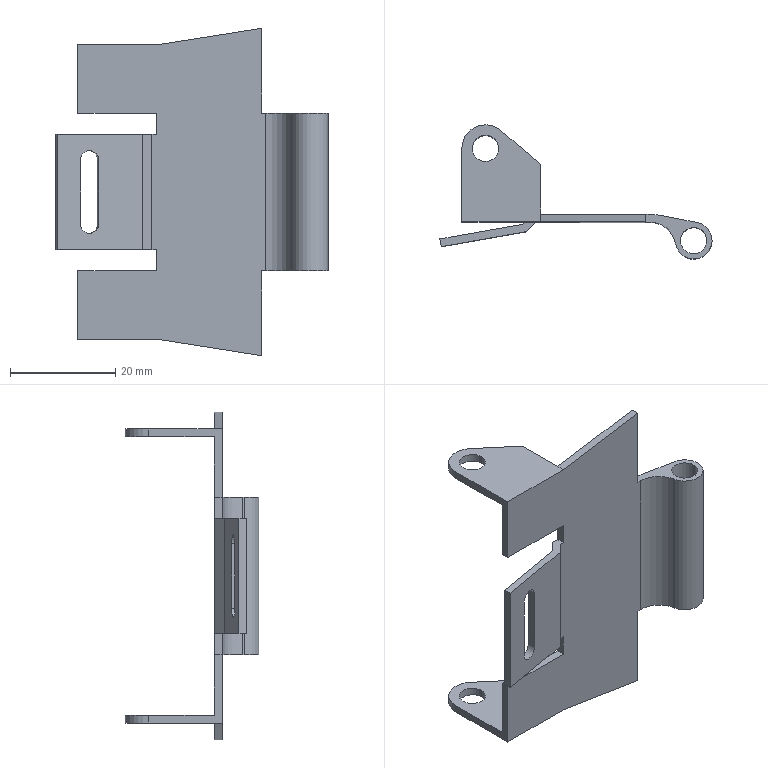Part | SolidWorks | features BaseBody 1 | 1 solid | 46 faces | box 51.82 x 25.52 x 62.335 mm | volume 4576 mm3 | plane 33 | cylinder 13 | commonest cylinder face diameters 5 x6 3.5 x2 9 x2 7 x1 10 x1 20 x1
STEP:
#1=CARTESIAN_POINT('',(2.5,0.,-1.5));
#2=VERTEX_POINT('',#1);
#3=CARTESIAN_POINT('',(-2.5,0.,-1.5));
#4=VERTEX_POINT('',#3);
#5=CARTESIAN_POINT('',(0.,0.,-1.5));
#6=DIRECTION('',(0.,0.,-1.));
#7=DIRECTION('',(1.,0.,0.));
#8=AXIS2_PLACEMENT_3D('',#5,#6,#7);
#9=CIRCLE('',#8,2.5);
#10=EDGE_CURVE('',#2,#4,#9,.T.);
#11=ORIENTED_EDGE('',*,*,#10,.T.);
#12=CARTESIAN_POINT('',(-2.5,0.,0.));
#13=VERTEX_POINT('',#12);
#14=CARTESIAN_POINT('',(-2.5,0.,-1.5));
#15=DIRECTION('',(0.,0.,1.));
#16=VECTOR('',#15,1000.);
#17=LINE('',#14,#16);
#18=EDGE_CURVE('',#4,#13,#17,.T.);
#19=ORIENTED_EDGE('',*,*,#18,.T.);
#20=CARTESIAN_POINT('',(2.5,0.,0.));
#21=VERTEX_POINT('',#20);
#22=CARTESIAN_POINT('',(0.,0.,0.));
#23=DIRECTION('',(0.,0.,-1.));
#24=DIRECTION('',(1.,0.,0.));
#25=AXIS2_PLACEMENT_3D('',#22,#23,#24);
#26=CIRCLE('',#25,2.5);
#27=EDGE_CURVE('',#21,#13,#26,.T.);
#28=ORIENTED_EDGE('',*,*,#27,.F.);
#29=CARTESIAN_POINT('',(2.5,0.,-1.5));
#30=DIRECTION('',(0.,0.,1.));
#31=VECTOR('',#30,1000.);
#32=LINE('',#29,#31);
#33=EDGE_CURVE('',#2,#21,#32,.T.);
#34=ORIENTED_EDGE('',*,*,#33,.F.);
#35=EDGE_LOOP('',(#11,#19,#28,#34));
#36=FACE_OUTER_BOUND('',#35,.T.);
#37=CARTESIAN_POINT('',(0.,0.,-1.5));
#38=DIRECTION('',(0.,0.,1.));
#39=DIRECTION('',(1.,0.,0.));
#40=AXIS2_PLACEMENT_3D('',#37,#38,#39);
#41=CYLINDRICAL_SURFACE('',#40,2.5);
#42=ADVANCED_FACE('',(#36),#41,.F.);
#43=CARTESIAN_POINT('',(2.5,0.,-54.5));
#44=VERTEX_POINT('',#43);
#45=CARTESIAN_POINT('',(-2.5,0.,-54.5));
#46=VERTEX_POINT('',#45);
#47=CARTESIAN_POINT('',(0.,0.,-54.5));
#48=DIRECTION('',(0.,0.,-1.));
#49=DIRECTION('',(-1.,0.,0.));
#50=AXIS2_PLACEMENT_3D('',#47,#48,#49);
#51=CIRCLE('',#50,2.5);
#52=EDGE_CURVE('',#44,#46,#51,.T.);
#53=ORIENTED_EDGE('',*,*,#52,.F.);
#54=CARTESIAN_POINT('',(2.5,0.,-56.));
#55=VERTEX_POINT('',#54);
#56=CARTESIAN_POINT('',(2.5,0.,-54.5));
#57=DIRECTION('',(0.,0.,-1.));
#58=VECTOR('',#57,1000.);
#59=LINE('',#56,#58);
#60=EDGE_CURVE('',#44,#55,#59,.T.);
#61=ORIENTED_EDGE('',*,*,#60,.T.);
#62=CARTESIAN_POINT('',(-2.5,0.,-56.));
#63=VERTEX_POINT('',#62);
#64=CARTESIAN_POINT('',(0.,0.,-56.));
#65=DIRECTION('',(0.,0.,1.));
#66=DIRECTION('',(-1.,0.,0.));
#67=AXIS2_PLACEMENT_3D('',#64,#65,#66);
#68=CIRCLE('',#67,2.5);
#69=EDGE_CURVE('',#63,#55,#68,.T.);
#70=ORIENTED_EDGE('',*,*,#69,.F.);
#71=CARTESIAN_POINT('',(-2.5,0.,-54.5));
#72=DIRECTION('',(0.,0.,-1.));
#73=VECTOR('',#72,1000.);
#74=LINE('',#71,#73);
#75=EDGE_CURVE('',#46,#63,#74,.T.);
#76=ORIENTED_EDGE('',*,*,#75,.F.);
#77=EDGE_LOOP('',(#53,#61,#70,#76));
#78=FACE_OUTER_BOUND('',#77,.T.);
#79=CARTESIAN_POINT('',(0.,0.,-54.5));
#80=DIRECTION('',(0.,0.,-1.));
#81=DIRECTION('',(-1.,0.,0.));
#82=AXIS2_PLACEMENT_3D('',#79,#80,#81);
#83=CYLINDRICAL_SURFACE('',#82,2.5);
#84=ADVANCED_FACE('',(#78),#83,.F.);
#85=CARTESIAN_POINT('',(37.15,-17.52,-13.));
#86=VERTEX_POINT('',#85);
#87=CARTESIAN_POINT('',(42.15,-17.52,-13.));
#88=VERTEX_POINT('',#87);
#89=CARTESIAN_POINT('',(39.65,-17.52,-13.));
#90=DIRECTION('',(0.,0.,1.));
#91=DIRECTION('',(-1.,0.,0.));
#92=AXIS2_PLACEMENT_3D('',#89,#90,#91);
#93=CIRCLE('',#92,2.5);
#94=EDGE_CURVE('',#86,#88,#93,.T.);
#95=ORIENTED_EDGE('',*,*,#94,.T.);
#96=CARTESIAN_POINT('',(42.15,-17.52,-43.));
#97=VERTEX_POINT('',#96);
#98=CARTESIAN_POINT('',(42.15,-17.52,-13.));
#99=DIRECTION('',(0.,0.,-1.));
#100=VECTOR('',#99,1000.);
#101=LINE('',#98,#100);
#102=EDGE_CURVE('',#88,#97,#101,.T.);
#103=ORIENTED_EDGE('',*,*,#102,.T.);
#104=CARTESIAN_POINT('',(37.15,-17.52,-43.));
#105=VERTEX_POINT('',#104);
#106=CARTESIAN_POINT('',(39.65,-17.52,-43.));
#107=DIRECTION('',(0.,0.,1.));
#108=DIRECTION('',(-1.,0.,0.));
#109=AXIS2_PLACEMENT_3D('',#106,#107,#108);
#110=CIRCLE('',#109,2.5);
#111=EDGE_CURVE('',#105,#97,#110,.T.);
#112=ORIENTED_EDGE('',*,*,#111,.F.);
#113=CARTESIAN_POINT('',(37.15,-17.52,-13.));
#114=DIRECTION('',(0.,0.,-1.));
#115=VECTOR('',#114,1000.);
#116=LINE('',#113,#115);
#117=EDGE_CURVE('',#86,#105,#116,.T.);
#118=ORIENTED_EDGE('',*,*,#117,.F.);
#119=EDGE_LOOP('',(#95,#103,#112,#118));
#120=FACE_OUTER_BOUND('',#119,.T.);
#121=CARTESIAN_POINT('',(39.65,-17.52,-13.));
#122=DIRECTION('',(0.,0.,-1.));
#123=DIRECTION('',(-1.,0.,0.));
#124=AXIS2_PLACEMENT_3D('',#121,#122,#123);
#125=CYLINDRICAL_SURFACE('',#124,2.5);
#126=ADVANCED_FACE('',(#120),#125,.F.);
#127=CARTESIAN_POINT('',(10.5,-14.,-17.));
#128=VERTEX_POINT('',#127);
#129=CARTESIAN_POINT('',(9.621,-14.,-17.));
#130=VERTEX_POINT('',#129);
#131=CARTESIAN_POINT('',(0.,-14.,-17.));
#132=DIRECTION('',(-1.,0.,0.));
#133=VECTOR('',#132,1000.);
#134=LINE('',#131,#133);
#135=EDGE_CURVE('',#128,#130,#134,.T.);
#136=ORIENTED_EDGE('',*,*,#135,.T.);
#137=CARTESIAN_POINT('',(9.621,-14.,-39.));
#138=VERTEX_POINT('',#137);
#139=CARTESIAN_POINT('',(9.621,-14.,-1.5));
#140=DIRECTION('',(0.,0.,-1.));
#141=VECTOR('',#140,1000.);
#142=LINE('',#139,#141);
#143=EDGE_CURVE('',#130,#138,#142,.T.);
#144=ORIENTED_EDGE('',*,*,#143,.T.);
#145=CARTESIAN_POINT('',(10.5,-14.,-39.));
#146=VERTEX_POINT('',#145);
#147=CARTESIAN_POINT('',(0.,-14.,-39.));
#148=DIRECTION('',(-1.,0.,0.));
#149=VECTOR('',#148,1000.);
#150=LINE('',#147,#149);
#151=EDGE_CURVE('',#146,#138,#150,.T.);
#152=ORIENTED_EDGE('',*,*,#151,.F.);
#153=CARTESIAN_POINT('',(10.5,-14.,-43.));
#154=VERTEX_POINT('',#153);
#155=CARTESIAN_POINT('',(10.5,-14.,-1.5));
#156=DIRECTION('',(0.,0.,-1.));
#157=VECTOR('',#156,1000.);
#158=LINE('',#155,#157);
#159=EDGE_CURVE('',#146,#154,#158,.T.);
#160=ORIENTED_EDGE('',*,*,#159,.T.);
#161=CARTESIAN_POINT('',(-4.5,-14.,-43.));
#162=VERTEX_POINT('',#161);
#163=CARTESIAN_POINT('',(-4.5,-14.,-43.));
#164=DIRECTION('',(-1.,0.,0.));
#165=VECTOR('',#164,1000.);
#166=LINE('',#163,#165);
#167=EDGE_CURVE('',#154,#162,#166,.T.);
#168=ORIENTED_EDGE('',*,*,#167,.T.);
#169=CARTESIAN_POINT('',(-4.5,-14.,-56.));
#170=VERTEX_POINT('',#169);
#171=CARTESIAN_POINT('',(-4.5,-14.,-1.5));
#172=DIRECTION('',(0.,0.,-1.));
#173=VECTOR('',#172,1000.);
#174=LINE('',#171,#173);
#175=EDGE_CURVE('',#162,#170,#174,.T.);
#176=ORIENTED_EDGE('',*,*,#175,.T.);
#177=CARTESIAN_POINT('',(10.5,-14.,-56.));
#178=VERTEX_POINT('',#177);
#179=CARTESIAN_POINT('',(-4.5,-14.,-56.));
#180=DIRECTION('',(1.,0.,0.));
#181=VECTOR('',#180,1000.);
#182=LINE('',#179,#181);
#183=EDGE_CURVE('',#170,#178,#182,.T.);
#184=ORIENTED_EDGE('',*,*,#183,.T.);
#185=CARTESIAN_POINT('',(30.5,-14.,-59.168));
#186=VERTEX_POINT('',#185);
#187=CARTESIAN_POINT('',(10.5,-14.,-56.));
#188=DIRECTION('',(0.9877,0.,-0.1564));
#189=VECTOR('',#188,1000.);
#190=LINE('',#187,#189);
#191=EDGE_CURVE('',#178,#186,#190,.T.);
#192=ORIENTED_EDGE('',*,*,#191,.T.);
#193=CARTESIAN_POINT('',(30.5,-14.,-43.));
#194=VERTEX_POINT('',#193);
#195=CARTESIAN_POINT('',(30.5,-14.,-1.5));
#196=DIRECTION('',(0.,0.,1.));
#197=VECTOR('',#196,1000.);
#198=LINE('',#195,#197);
#199=EDGE_CURVE('',#186,#194,#198,.T.);
#200=ORIENTED_EDGE('',*,*,#199,.T.);
#201=CARTESIAN_POINT('',(31.271,-14.,-43.));
#202=VERTEX_POINT('',#201);
#203=CARTESIAN_POINT('',(31.202,-14.,-43.));
#204=DIRECTION('',(-1.,0.,0.));
#205=VECTOR('',#204,1000.);
#206=LINE('',#203,#205);
#207=EDGE_CURVE('',#202,#194,#206,.T.);
#208=ORIENTED_EDGE('',*,*,#207,.F.);
#209=CARTESIAN_POINT('',(31.271,-14.,-13.));
#210=VERTEX_POINT('',#209);
#211=CARTESIAN_POINT('',(31.271,-14.,-1.5));
#212=DIRECTION('',(0.,0.,1.));
#213=VECTOR('',#212,1000.);
#214=LINE('',#211,#213);
#215=EDGE_CURVE('',#202,#210,#214,.T.);
#216=ORIENTED_EDGE('',*,*,#215,.T.);
#217=CARTESIAN_POINT('',(30.5,-14.,-13.));
#218=VERTEX_POINT('',#217);
#219=CARTESIAN_POINT('',(31.202,-14.,-13.));
#220=DIRECTION('',(-1.,0.,0.));
#221=VECTOR('',#220,1000.);
#222=LINE('',#219,#221);
#223=EDGE_CURVE('',#210,#218,#222,.T.);
#224=ORIENTED_EDGE('',*,*,#223,.T.);
#225=CARTESIAN_POINT('',(30.5,-14.,3.168));
#226=VERTEX_POINT('',#225);
#227=CARTESIAN_POINT('',(30.5,-14.,-1.5));
#228=DIRECTION('',(0.,0.,1.));
#229=VECTOR('',#228,1000.);
#230=LINE('',#227,#229);
#231=EDGE_CURVE('',#218,#226,#230,.T.);
#232=ORIENTED_EDGE('',*,*,#231,.T.);
#233=CARTESIAN_POINT('',(10.5,-14.,0.));
#234=VERTEX_POINT('',#233);
#235=CARTESIAN_POINT('',(30.5,-14.,3.168));
#236=DIRECTION('',(-0.9877,0.,-0.1564));
#237=VECTOR('',#236,1000.);
#238=LINE('',#235,#237);
#239=EDGE_CURVE('',#226,#234,#238,.T.);
#240=ORIENTED_EDGE('',*,*,#239,.T.);
#241=CARTESIAN_POINT('',(-4.5,-14.,0.));
#242=VERTEX_POINT('',#241);
#243=CARTESIAN_POINT('',(-4.5,-14.,0.));
#244=DIRECTION('',(-1.,0.,0.));
#245=VECTOR('',#244,1000.);
#246=LINE('',#243,#245);
#247=EDGE_CURVE('',#234,#242,#246,.T.);
#248=ORIENTED_EDGE('',*,*,#247,.T.);
#249=CARTESIAN_POINT('',(-4.5,-14.,-13.));
#250=VERTEX_POINT('',#249);
#251=CARTESIAN_POINT('',(-4.5,-14.,-1.5));
#252=DIRECTION('',(0.,0.,-1.));
#253=VECTOR('',#252,1000.);
#254=LINE('',#251,#253);
#255=EDGE_CURVE('',#242,#250,#254,.T.);
#256=ORIENTED_EDGE('',*,*,#255,.T.);
#257=CARTESIAN_POINT('',(10.5,-14.,-13.));
#258=VERTEX_POINT('',#257);
#259=CARTESIAN_POINT('',(-4.5,-14.,-13.));
#260=DIRECTION('',(1.,0.,0.));
#261=VECTOR('',#260,1000.);
#262=LINE('',#259,#261);
#263=EDGE_CURVE('',#250,#258,#262,.T.);
#264=ORIENTED_EDGE('',*,*,#263,.T.);
#265=CARTESIAN_POINT('',(10.5,-14.,-1.5));
#266=DIRECTION('',(0.,0.,-1.));
#267=VECTOR('',#266,1000.);
#268=LINE('',#265,#267);
#269=EDGE_CURVE('',#258,#128,#268,.T.);
#270=ORIENTED_EDGE('',*,*,#269,.T.);
#271=EDGE_LOOP('',(#136,#144,#152,#160,#168,#176,#184,#192,#200,#208,#216,#224,#232,#240,#248,#256,#264,#270));
#272=FACE_OUTER_BOUND('',#271,.T.);
#273=CARTESIAN_POINT('',(-4.5,-14.,-1.5));
#274=DIRECTION('',(0.,-1.,0.));
#275=DIRECTION('',(0.,0.,-1.));
#276=AXIS2_PLACEMENT_3D('',#273,#274,#275);
#277=PLANE('',#276);
#278=ADVANCED_FACE('',(#272),#277,.T.);
#279=CARTESIAN_POINT('',(7.813,-15.808,-17.));
#280=VERTEX_POINT('',#279);
#281=CARTESIAN_POINT('',(9.621,-14.,-17.));
#282=DIRECTION('',(0.7071,0.7071,0.));
#283=VECTOR('',#282,1000.);
#284=LINE('',#281,#283);
#285=EDGE_CURVE('',#280,#130,#284,.T.);
#286=ORIENTED_EDGE('',*,*,#285,.F.);
#287=CARTESIAN_POINT('',(7.813,-15.808,-39.));
#288=VERTEX_POINT('',#287);
#289=CARTESIAN_POINT('',(7.813,-15.808,-17.));
#290=DIRECTION('',(0.,0.,1.));
#291=VECTOR('',#290,1000.);
#292=LINE('',#289,#291);
#293=EDGE_CURVE('',#288,#280,#292,.T.);
#294=ORIENTED_EDGE('',*,*,#293,.F.);
#295=CARTESIAN_POINT('',(9.621,-14.,-39.));
#296=DIRECTION('',(-0.7071,-0.7071,0.));
#297=VECTOR('',#296,1000.);
#298=LINE('',#295,#297);
#299=EDGE_CURVE('',#138,#288,#298,.T.);
#300=ORIENTED_EDGE('',*,*,#299,.F.);
#301=ORIENTED_EDGE('',*,*,#143,.F.);
#302=EDGE_LOOP('',(#286,#294,#300,#301));
#303=FACE_OUTER_BOUND('',#302,.T.);
#304=CARTESIAN_POINT('',(9.621,-14.,-17.));
#305=DIRECTION('',(-0.7071,0.7071,0.));
#306=DIRECTION('',(-0.7071,-0.7071,0.));
#307=AXIS2_PLACEMENT_3D('',#304,#305,#306);
#308=PLANE('',#307);
#309=ADVANCED_FACE('',(#303),#308,.F.);
#310=CARTESIAN_POINT('',(10.5,-12.5,-13.));
#311=VERTEX_POINT('',#310);
#312=CARTESIAN_POINT('',(10.5,-14.,-13.));
#313=DIRECTION('',(0.,-1.,0.));
#314=VECTOR('',#313,1000.);
#315=LINE('',#312,#314);
#316=EDGE_CURVE('',#311,#258,#315,.T.);
#317=ORIENTED_EDGE('',*,*,#316,.F.);
#318=CARTESIAN_POINT('',(10.5,-12.5,-17.));
#319=VERTEX_POINT('',#318);
#320=CARTESIAN_POINT('',(10.5,-12.5,-43.));
#321=DIRECTION('',(0.,0.,1.));
#322=VECTOR('',#321,1000.);
#323=LINE('',#320,#322);
#324=EDGE_CURVE('',#319,#311,#323,.T.);
#325=ORIENTED_EDGE('',*,*,#324,.F.);
#326=CARTESIAN_POINT('',(10.5,-14.,-17.));
#327=DIRECTION('',(0.,1.,0.));
#328=VECTOR('',#327,1000.);
#329=LINE('',#326,#328);
#330=EDGE_CURVE('',#128,#319,#329,.T.);
#331=ORIENTED_EDGE('',*,*,#330,.F.);
#332=ORIENTED_EDGE('',*,*,#269,.F.);
#333=EDGE_LOOP('',(#317,#325,#331,#332));
#334=FACE_OUTER_BOUND('',#333,.T.);
#335=CARTESIAN_POINT('',(10.5,-14.,-43.));
#336=DIRECTION('',(1.,0.,0.));
#337=DIRECTION('',(0.,0.,-1.));
#338=AXIS2_PLACEMENT_3D('',#335,#336,#337);
#339=PLANE('',#338);
#340=ADVANCED_FACE('',(#334),#339,.F.);
#341=ORIENTED_EDGE('',*,*,#263,.F.);
#342=CARTESIAN_POINT('',(-4.5,-12.5,-13.));
#343=VERTEX_POINT('',#342);
#344=CARTESIAN_POINT('',(-4.5,-14.,-13.));
#345=DIRECTION('',(0.,-1.,0.));
#346=VECTOR('',#345,1000.);
#347=LINE('',#344,#346);
#348=EDGE_CURVE('',#343,#250,#347,.T.);
#349=ORIENTED_EDGE('',*,*,#348,.F.);
#350=CARTESIAN_POINT('',(-4.5,-12.5,-13.));
#351=DIRECTION('',(-1.,0.,0.));
#352=VECTOR('',#351,1000.);
#353=LINE('',#350,#352);
#354=EDGE_CURVE('',#311,#343,#353,.T.);
#355=ORIENTED_EDGE('',*,*,#354,.F.);
#356=ORIENTED_EDGE('',*,*,#316,.T.);
#357=EDGE_LOOP('',(#341,#349,#355,#356));
#358=FACE_OUTER_BOUND('',#357,.T.);
#359=CARTESIAN_POINT('',(-4.5,-14.,-13.));
#360=DIRECTION('',(0.,0.,1.));
#361=DIRECTION('',(1.,0.,0.));
#362=AXIS2_PLACEMENT_3D('',#359,#360,#361);
#363=PLANE('',#362);
#364=ADVANCED_FACE('',(#358),#363,.F.);
#365=CARTESIAN_POINT('',(-4.5,0.,0.));
#366=VERTEX_POINT('',#365);
#367=CARTESIAN_POINT('',(-4.5,0.,0.));
#368=DIRECTION('',(0.,1.,0.));
#369=VECTOR('',#368,1000.);
#370=LINE('',#367,#369);
#371=EDGE_CURVE('',#242,#366,#370,.T.);
#372=ORIENTED_EDGE('',*,*,#371,.T.);
#373=CARTESIAN_POINT('',(-4.5,0.,-1.5));
#374=VERTEX_POINT('',#373);
#375=CARTESIAN_POINT('',(-4.5,0.,-1.5));
#376=DIRECTION('',(0.,0.,1.));
#377=VECTOR('',#376,1000.);
#378=LINE('',#375,#377);
#379=EDGE_CURVE('',#374,#366,#378,.T.);
#380=ORIENTED_EDGE('',*,*,#379,.F.);
#381=CARTESIAN_POINT('',(-4.5,-12.5,-1.5));
#382=VERTEX_POINT('',#381);
#383=CARTESIAN_POINT('',(-4.5,0.,-1.5));
#384=DIRECTION('',(0.,-1.,0.));
#385=VECTOR('',#384,1000.);
#386=LINE('',#383,#385);
#387=EDGE_CURVE('',#374,#382,#386,.T.);
#388=ORIENTED_EDGE('',*,*,#387,.T.);
#389=CARTESIAN_POINT('',(-4.5,-12.5,-1.5));
#390=DIRECTION('',(0.,0.,-1.));
#391=VECTOR('',#390,1000.);
#392=LINE('',#389,#391);
#393=EDGE_CURVE('',#382,#343,#392,.T.);
#394=ORIENTED_EDGE('',*,*,#393,.T.);
#395=ORIENTED_EDGE('',*,*,#348,.T.);
#396=ORIENTED_EDGE('',*,*,#255,.F.);
#397=EDGE_LOOP('',(#372,#380,#388,#394,#395,#396));
#398=FACE_OUTER_BOUND('',#397,.T.);
#399=CARTESIAN_POINT('',(-4.5,0.,-1.5));
#400=DIRECTION('',(-1.,0.,0.));
#401=DIRECTION('',(0.,-1.,0.));
#402=AXIS2_PLACEMENT_3D('',#399,#400,#401);
#403=PLANE('',#402);
#404=ADVANCED_FACE('',(#398),#403,.T.);
#405=ORIENTED_EDGE('',*,*,#27,.T.);
#406=CARTESIAN_POINT('',(0.,0.,0.));
#407=DIRECTION('',(0.,0.,-1.));
#408=DIRECTION('',(1.,0.,0.));
#409=AXIS2_PLACEMENT_3D('',#406,#407,#408);
#410=CIRCLE('',#409,2.5);
#411=EDGE_CURVE('',#13,#21,#410,.T.);
#412=ORIENTED_EDGE('',*,*,#411,.T.);
#413=EDGE_LOOP('',(#405,#412));
#414=FACE_BOUND('',#413,.T.);
#415=ORIENTED_EDGE('',*,*,#247,.F.);
#416=CARTESIAN_POINT('',(10.5,-12.5,0.));
#417=VERTEX_POINT('',#416);
#418=CARTESIAN_POINT('',(10.5,0.,0.));
#419=DIRECTION('',(0.,1.,0.));
#420=VECTOR('',#419,1000.);
#421=LINE('',#418,#420);
#422=EDGE_CURVE('',#234,#417,#421,.T.);
#423=ORIENTED_EDGE('',*,*,#422,.T.);
#424=CARTESIAN_POINT('',(10.5,-3.,0.));
#425=VERTEX_POINT('',#424);
#426=CARTESIAN_POINT('',(10.5,0.,0.));
#427=DIRECTION('',(0.,1.,0.));
#428=VECTOR('',#427,1000.);
#429=LINE('',#426,#428);
#430=EDGE_CURVE('',#417,#425,#429,.T.);
#431=ORIENTED_EDGE('',*,*,#430,.T.);
#432=CARTESIAN_POINT('',(2.909,3.433,0.));
#433=VERTEX_POINT('',#432);
#434=CARTESIAN_POINT('',(10.5,-3.,0.));
#435=DIRECTION('',(-0.7629,0.6465,0.));
#436=VECTOR('',#435,1000.);
#437=LINE('',#434,#436);
#438=EDGE_CURVE('',#425,#433,#437,.T.);
#439=ORIENTED_EDGE('',*,*,#438,.T.);
#440=CARTESIAN_POINT('',(0.,0.,0.));
#441=DIRECTION('',(0.,0.,1.));
#442=DIRECTION('',(1.,0.,0.));
#443=AXIS2_PLACEMENT_3D('',#440,#441,#442);
#444=CIRCLE('',#443,4.5);
#445=EDGE_CURVE('',#433,#366,#444,.T.);
#446=ORIENTED_EDGE('',*,*,#445,.T.);
#447=ORIENTED_EDGE('',*,*,#371,.F.);
#448=EDGE_LOOP('',(#415,#423,#431,#439,#446,#447));
#449=FACE_OUTER_BOUND('',#448,.T.);
#450=CARTESIAN_POINT('',(0.,0.,0.));
#451=DIRECTION('',(0.,0.,1.));
#452=DIRECTION('',(1.,0.,0.));
#453=AXIS2_PLACEMENT_3D('',#450,#451,#452);
#454=PLANE('',#453);
#455=ADVANCED_FACE('',(#414,#449),#454,.T.);
#456=ORIENTED_EDGE('',*,*,#239,.F.);
#457=CARTESIAN_POINT('',(30.5,-12.5,3.168));
#458=VERTEX_POINT('',#457);
#459=CARTESIAN_POINT('',(30.5,-12.5,3.168));
#460=DIRECTION('',(0.,1.,0.));
#461=VECTOR('',#460,1000.);
#462=LINE('',#459,#461);
#463=EDGE_CURVE('',#226,#458,#462,.T.);
#464=ORIENTED_EDGE('',*,*,#463,.T.);
#465=CARTESIAN_POINT('',(10.5,-12.5,0.));
#466=DIRECTION('',(-0.9877,0.,-0.1564));
#467=VECTOR('',#466,1000.);
#468=LINE('',#465,#467);
#469=EDGE_CURVE('',#458,#417,#468,.T.);
#470=ORIENTED_EDGE('',*,*,#469,.T.);
#471=ORIENTED_EDGE('',*,*,#422,.F.);
#472=EDGE_LOOP('',(#456,#464,#470,#471));
#473=FACE_OUTER_BOUND('',#472,.T.);
#474=CARTESIAN_POINT('',(10.5,-12.5,0.));
#475=DIRECTION('',(-0.1564,0.,0.9877));
#476=DIRECTION('',(0.9877,0.,0.1564));
#477=AXIS2_PLACEMENT_3D('',#474,#475,#476);
#478=PLANE('',#477);
#479=ADVANCED_FACE('',(#473),#478,.T.);
#480=CARTESIAN_POINT('',(30.5,-12.5,-13.));
#481=VERTEX_POINT('',#480);
#482=CARTESIAN_POINT('',(30.5,-22.5,-13.));
#483=DIRECTION('',(0.,1.,0.));
#484=VECTOR('',#483,1000.);
#485=LINE('',#482,#484);
#486=EDGE_CURVE('',#218,#481,#485,.T.);
#487=ORIENTED_EDGE('',*,*,#486,.T.);
#488=CARTESIAN_POINT('',(30.5,-12.5,3.168));
#489=DIRECTION('',(0.,0.,1.));
#490=VECTOR('',#489,1000.);
#491=LINE('',#488,#490);
#492=EDGE_CURVE('',#481,#458,#491,.T.);
#493=ORIENTED_EDGE('',*,*,#492,.T.);
#494=ORIENTED_EDGE('',*,*,#463,.F.);
#495=ORIENTED_EDGE('',*,*,#231,.F.);
#496=EDGE_LOOP('',(#487,#493,#494,#495));
#497=FACE_OUTER_BOUND('',#496,.T.);
#498=CARTESIAN_POINT('',(30.5,-12.5,3.168));
#499=DIRECTION('',(1.,0.,0.));
#500=DIRECTION('',(0.,0.,-1.));
#501=AXIS2_PLACEMENT_3D('',#498,#499,#500);
#502=PLANE('',#501);
#503=ADVANCED_FACE('',(#497),#502,.T.);
#504=CARTESIAN_POINT('',(36.152,-17.915,-13.));
#505=VERTEX_POINT('',#504);
#506=CARTESIAN_POINT('',(31.271,-19.,-13.));
#507=DIRECTION('',(0.,0.,-1.));
#508=DIRECTION('',(-1.,0.,0.));
#509=AXIS2_PLACEMENT_3D('',#506,#507,#508);
#510=CIRCLE('',#509,5.);
#511=EDGE_CURVE('',#210,#505,#510,.T.);
#512=ORIENTED_EDGE('',*,*,#511,.F.);
#513=ORIENTED_EDGE('',*,*,#215,.F.);
#514=CARTESIAN_POINT('',(36.152,-17.915,-43.));
#515=VERTEX_POINT('',#514);
#516=CARTESIAN_POINT('',(31.271,-19.,-43.));
#517=DIRECTION('',(0.,0.,1.));
#518=DIRECTION('',(-1.,0.,0.));
#519=AXIS2_PLACEMENT_3D('',#516,#517,#518);
#520=CIRCLE('',#519,5.);
#521=EDGE_CURVE('',#515,#202,#520,.T.);
#522=ORIENTED_EDGE('',*,*,#521,.F.);
#523=CARTESIAN_POINT('',(36.152,-17.915,-13.));
#524=DIRECTION('',(0.,0.,-1.));
#525=VECTOR('',#524,1000.);
#526=LINE('',#523,#525);
#527=EDGE_CURVE('',#505,#515,#526,.T.);
#528=ORIENTED_EDGE('',*,*,#527,.F.);
#529=EDGE_LOOP('',(#512,#513,#522,#528));
#530=FACE_OUTER_BOUND('',#529,.T.);
#531=CARTESIAN_POINT('',(31.271,-19.,-13.));
#532=DIRECTION('',(0.,0.,-1.));
#533=DIRECTION('',(-1.,0.,0.));
#534=AXIS2_PLACEMENT_3D('',#531,#532,#533);
#535=CYLINDRICAL_SURFACE('',#534,5.);
#536=ADVANCED_FACE('',(#530),#535,.F.);
#537=CARTESIAN_POINT('',(30.5,-12.5,-59.168));
#538=VERTEX_POINT('',#537);
#539=CARTESIAN_POINT('',(30.5,-12.5,-43.));
#540=VERTEX_POINT('',#539);
#541=CARTESIAN_POINT('',(30.5,-12.5,3.168));
#542=DIRECTION('',(0.,0.,1.));
#543=VECTOR('',#542,1000.);
#544=LINE('',#541,#543);
#545=EDGE_CURVE('',#538,#540,#544,.T.);
#546=ORIENTED_EDGE('',*,*,#545,.T.);
#547=CARTESIAN_POINT('',(30.5,-12.5,-43.));
#548=DIRECTION('',(0.,-1.,0.));
#549=VECTOR('',#548,1000.);
#550=LINE('',#547,#549);
#551=EDGE_CURVE('',#540,#194,#550,.T.);
#552=ORIENTED_EDGE('',*,*,#551,.T.);
#553=ORIENTED_EDGE('',*,*,#199,.F.);
#554=CARTESIAN_POINT('',(30.5,-12.5,-59.168));
#555=DIRECTION('',(0.,1.,0.));
#556=VECTOR('',#555,1000.);
#557=LINE('',#554,#556);
#558=EDGE_CURVE('',#186,#538,#557,.T.);
#559=ORIENTED_EDGE('',*,*,#558,.T.);
#560=EDGE_LOOP('',(#546,#552,#553,#559));
#561=FACE_OUTER_BOUND('',#560,.T.);
#562=CARTESIAN_POINT('',(30.5,-12.5,3.168));
#563=DIRECTION('',(1.,0.,0.));
#564=DIRECTION('',(0.,0.,-1.));
#565=AXIS2_PLACEMENT_3D('',#562,#563,#564);
#566=PLANE('',#565);
#567=ADVANCED_FACE('',(#561),#566,.T.);
#568=ORIENTED_EDGE('',*,*,#191,.F.);
#569=CARTESIAN_POINT('',(10.5,-12.5,-56.));
#570=VERTEX_POINT('',#569);
#571=CARTESIAN_POINT('',(10.5,-12.5,-56.));
#572=DIRECTION('',(0.,1.,0.));
#573=VECTOR('',#572,1000.);
#574=LINE('',#571,#573);
#575=EDGE_CURVE('',#178,#570,#574,.T.);
#576=ORIENTED_EDGE('',*,*,#575,.T.);
#577=CARTESIAN_POINT('',(10.5,-12.5,-56.));
#578=DIRECTION('',(0.9877,0.,-0.1564));
#579=VECTOR('',#578,1000.);
#580=LINE('',#577,#579);
#581=EDGE_CURVE('',#570,#538,#580,.T.);
#582=ORIENTED_EDGE('',*,*,#581,.T.);
#583=ORIENTED_EDGE('',*,*,#558,.F.);
#584=EDGE_LOOP('',(#568,#576,#582,#583));
#585=FACE_OUTER_BOUND('',#584,.T.);
#586=CARTESIAN_POINT('',(10.5,-12.5,-56.));
#587=DIRECTION('',(-0.1564,0.,-0.9877));
#588=DIRECTION('',(-0.9877,0.,0.1564));
#589=AXIS2_PLACEMENT_3D('',#586,#587,#588);
#590=PLANE('',#589);
#591=ADVANCED_FACE('',(#585),#590,.T.);
#592=CARTESIAN_POINT('',(-4.5,0.,-56.));
#593=VERTEX_POINT('',#592);
#594=CARTESIAN_POINT('',(2.909,3.433,-56.));
#595=VERTEX_POINT('',#594);
#596=CARTESIAN_POINT('',(0.,0.,-56.));
#597=DIRECTION('',(0.,0.,-1.));
#598=DIRECTION('',(-1.,0.,0.));
#599=AXIS2_PLACEMENT_3D('',#596,#597,#598);
#600=CIRCLE('',#599,4.5);
#601=EDGE_CURVE('',#593,#595,#600,.T.);
#602=ORIENTED_EDGE('',*,*,#601,.T.);
#603=CARTESIAN_POINT('',(10.5,-3.,-56.));
#604=VERTEX_POINT('',#603);
#605=CARTESIAN_POINT('',(2.909,3.433,-56.));
#606=DIRECTION('',(0.7629,-0.6465,0.));
#607=VECTOR('',#606,1000.);
#608=LINE('',#605,#607);
#609=EDGE_CURVE('',#595,#604,#608,.T.);
#610=ORIENTED_EDGE('',*,*,#609,.T.);
#611=CARTESIAN_POINT('',(10.5,-12.5,-56.));
#612=DIRECTION('',(0.,-1.,0.));
#613=VECTOR('',#612,1000.);
#614=LINE('',#611,#613);
#615=EDGE_CURVE('',#604,#570,#614,.T.);
#616=ORIENTED_EDGE('',*,*,#615,.T.);
#617=ORIENTED_EDGE('',*,*,#575,.F.);
#618=ORIENTED_EDGE('',*,*,#183,.F.);
#619=CARTESIAN_POINT('',(-4.5,-12.5,-56.));
#620=DIRECTION('',(0.,1.,0.));
#621=VECTOR('',#620,1000.);
#622=LINE('',#619,#621);
#623=EDGE_CURVE('',#170,#593,#622,.T.);
#624=ORIENTED_EDGE('',*,*,#623,.T.);
#625=EDGE_LOOP('',(#602,#610,#616,#617,#618,#624));
#626=FACE_OUTER_BOUND('',#625,.T.);
#627=ORIENTED_EDGE('',*,*,#69,.T.);
#628=CARTESIAN_POINT('',(0.,0.,-56.));
#629=DIRECTION('',(0.,0.,1.));
#630=DIRECTION('',(-1.,0.,0.));
#631=AXIS2_PLACEMENT_3D('',#628,#629,#630);
#632=CIRCLE('',#631,2.5);
#633=EDGE_CURVE('',#55,#63,#632,.T.);
#634=ORIENTED_EDGE('',*,*,#633,.T.);
#635=EDGE_LOOP('',(#627,#634));
#636=FACE_BOUND('',#635,.T.);
#637=CARTESIAN_POINT('',(10.5,-12.5,-56.));
#638=DIRECTION('',(0.,0.,-1.));
#639=DIRECTION('',(-1.,0.,0.));
#640=AXIS2_PLACEMENT_3D('',#637,#638,#639);
#641=PLANE('',#640);
#642=ADVANCED_FACE('',(#626,#636),#641,.T.);
#643=CARTESIAN_POINT('',(-4.5,-12.5,-54.5));
#644=VERTEX_POINT('',#643);
#645=CARTESIAN_POINT('',(-4.5,0.,-54.5));
#646=VERTEX_POINT('',#645);
#647=CARTESIAN_POINT('',(-4.5,0.,-54.5));
#648=DIRECTION('',(0.,1.,0.));
#649=VECTOR('',#648,1000.);
#650=LINE('',#647,#649);
#651=EDGE_CURVE('',#644,#646,#650,.T.);
#652=ORIENTED_EDGE('',*,*,#651,.T.);
#653=CARTESIAN_POINT('',(-4.5,0.,-1.5));
#654=DIRECTION('',(0.,0.,-1.));
#655=VECTOR('',#654,1000.);
#656=LINE('',#653,#655);
#657=EDGE_CURVE('',#646,#593,#656,.T.);
#658=ORIENTED_EDGE('',*,*,#657,.T.);
#659=ORIENTED_EDGE('',*,*,#623,.F.);
#660=ORIENTED_EDGE('',*,*,#175,.F.);
#661=CARTESIAN_POINT('',(-4.5,-12.5,-43.));
#662=VERTEX_POINT('',#661);
#663=CARTESIAN_POINT('',(-4.5,0.,-43.));
#664=DIRECTION('',(0.,1.,0.));
#665=VECTOR('',#664,1000.);
#666=LINE('',#663,#665);
#667=EDGE_CURVE('',#162,#662,#666,.T.);
#668=ORIENTED_EDGE('',*,*,#667,.T.);
#669=CARTESIAN_POINT('',(-4.5,-12.5,-1.5));
#670=DIRECTION('',(0.,0.,-1.));
#671=VECTOR('',#670,1000.);
#672=LINE('',#669,#671);
#673=EDGE_CURVE('',#662,#644,#672,.T.);
#674=ORIENTED_EDGE('',*,*,#673,.T.);
#675=EDGE_LOOP('',(#652,#658,#659,#660,#668,#674));
#676=FACE_OUTER_BOUND('',#675,.T.);
#677=CARTESIAN_POINT('',(-4.5,0.,-1.5));
#678=DIRECTION('',(-1.,0.,0.));
#679=DIRECTION('',(0.,-1.,0.));
#680=AXIS2_PLACEMENT_3D('',#677,#678,#679);
#681=PLANE('',#680);
#682=ADVANCED_FACE('',(#676),#681,.T.);
#683=ORIENTED_EDGE('',*,*,#167,.F.);
#684=CARTESIAN_POINT('',(10.5,-12.5,-43.));
#685=VERTEX_POINT('',#684);
#686=CARTESIAN_POINT('',(10.5,-14.,-43.));
#687=DIRECTION('',(0.,-1.,0.));
#688=VECTOR('',#687,1000.);
#689=LINE('',#686,#688);
#690=EDGE_CURVE('',#685,#154,#689,.T.);
#691=ORIENTED_EDGE('',*,*,#690,.F.);
#692=CARTESIAN_POINT('',(-4.5,-12.5,-43.));
#693=DIRECTION('',(1.,0.,0.));
#694=VECTOR('',#693,1000.);
#695=LINE('',#692,#694);
#696=EDGE_CURVE('',#662,#685,#695,.T.);
#697=ORIENTED_EDGE('',*,*,#696,.F.);
#698=ORIENTED_EDGE('',*,*,#667,.F.);
#699=EDGE_LOOP('',(#683,#691,#697,#698));
#700=FACE_OUTER_BOUND('',#699,.T.);
#701=CARTESIAN_POINT('',(-4.5,-14.,-43.));
#702=DIRECTION('',(0.,0.,-1.));
#703=DIRECTION('',(-1.,0.,0.));
#704=AXIS2_PLACEMENT_3D('',#701,#702,#703);
#705=PLANE('',#704);
#706=ADVANCED_FACE('',(#700),#705,.F.);
#707=CARTESIAN_POINT('',(10.5,-12.5,-39.));
#708=VERTEX_POINT('',#707);
#709=CARTESIAN_POINT('',(10.5,-12.5,-43.));
#710=DIRECTION('',(0.,0.,1.));
#711=VECTOR('',#710,1000.);
#712=LINE('',#709,#711);
#713=EDGE_CURVE('',#685,#708,#712,.T.);
#714=ORIENTED_EDGE('',*,*,#713,.F.);
#715=ORIENTED_EDGE('',*,*,#690,.T.);
#716=ORIENTED_EDGE('',*,*,#159,.F.);
#717=CARTESIAN_POINT('',(10.5,-14.,-39.));
#718=DIRECTION('',(0.,-1.,0.));
#719=VECTOR('',#718,1000.);
#720=LINE('',#717,#719);
#721=EDGE_CURVE('',#708,#146,#720,.T.);
#722=ORIENTED_EDGE('',*,*,#721,.F.);
#723=EDGE_LOOP('',(#714,#715,#716,#722));
#724=FACE_OUTER_BOUND('',#723,.T.);
#725=CARTESIAN_POINT('',(10.5,-14.,-43.));
#726=DIRECTION('',(1.,0.,0.));
#727=DIRECTION('',(0.,0.,-1.));
#728=AXIS2_PLACEMENT_3D('',#725,#726,#727);
#729=PLANE('',#728);
#730=ADVANCED_FACE('',(#724),#729,.F.);
#731=CARTESIAN_POINT('',(7.087,-14.413,-17.));
#732=VERTEX_POINT('',#731);
#733=CARTESIAN_POINT('',(9.,-12.5,-17.));
#734=VERTEX_POINT('',#733);
#735=CARTESIAN_POINT('',(7.087,-14.413,-17.));
#736=DIRECTION('',(0.7071,0.7071,0.));
#737=VECTOR('',#736,1000.);
#738=LINE('',#735,#737);
#739=EDGE_CURVE('',#732,#734,#738,.T.);
#740=ORIENTED_EDGE('',*,*,#739,.F.);
#741=CARTESIAN_POINT('',(-8.67,-17.191,-17.));
#742=VERTEX_POINT('',#741);
#743=CARTESIAN_POINT('',(-8.67,-17.191,-17.));
#744=DIRECTION('',(0.9848,0.1736,0.));
#745=VECTOR('',#744,1000.);
#746=LINE('',#743,#745);
#747=EDGE_CURVE('',#742,#732,#746,.T.);
#748=ORIENTED_EDGE('',*,*,#747,.F.);
#749=CARTESIAN_POINT('',(-8.409,-18.669,-17.));
#750=VERTEX_POINT('',#749);
#751=CARTESIAN_POINT('',(-8.67,-17.191,-17.));
#752=DIRECTION('',(0.1736,-0.9848,0.));
#753=VECTOR('',#752,1000.);
#754=LINE('',#751,#753);
#755=EDGE_CURVE('',#742,#750,#754,.T.);
#756=ORIENTED_EDGE('',*,*,#755,.T.);
#757=CARTESIAN_POINT('',(7.813,-15.808,-17.));
#758=DIRECTION('',(-0.9848,-0.1736,0.));
#759=VECTOR('',#758,1000.);
#760=LINE('',#757,#759);
#761=EDGE_CURVE('',#280,#750,#760,.T.);
#762=ORIENTED_EDGE('',*,*,#761,.F.);
#763=ORIENTED_EDGE('',*,*,#285,.T.);
#764=ORIENTED_EDGE('',*,*,#135,.F.);
#765=ORIENTED_EDGE('',*,*,#330,.T.);
#766=CARTESIAN_POINT('',(0.,-12.5,-17.));
#767=DIRECTION('',(1.,0.,0.));
#768=VECTOR('',#767,1000.);
#769=LINE('',#766,#768);
#770=EDGE_CURVE('',#734,#319,#769,.T.);
#771=ORIENTED_EDGE('',*,*,#770,.F.);
#772=EDGE_LOOP('',(#740,#748,#756,#762,#763,#764,#765,#771));
#773=FACE_OUTER_BOUND('',#772,.T.);
#774=CARTESIAN_POINT('',(0.,0.,-17.));
#775=DIRECTION('',(0.,0.,-1.));
#776=DIRECTION('',(-1.,0.,0.));
#777=AXIS2_PLACEMENT_3D('',#774,#775,#776);
#778=PLANE('',#777);
#779=ADVANCED_FACE('',(#773),#778,.F.);
#780=CARTESIAN_POINT('',(-3.978,-17.887,-21.875));
#781=VERTEX_POINT('',#780);
#782=CARTESIAN_POINT('',(-3.978,-17.887,-34.125));
#783=VERTEX_POINT('',#782);
#784=CARTESIAN_POINT('',(-3.978,-17.887,-17.));
#785=DIRECTION('',(0.,0.,-1.));
#786=VECTOR('',#785,1000.);
#787=LINE('',#784,#786);
#788=EDGE_CURVE('',#781,#783,#787,.T.);
#789=ORIENTED_EDGE('',*,*,#788,.F.);
#790=CARTESIAN_POINT('',(-0.531,-17.279,-21.875));
#791=VERTEX_POINT('',#790);
#792=CARTESIAN_POINT('',(-2.254,-17.583,-21.875));
#793=DIRECTION('',(0.1736,-0.9848,0.));
#794=DIRECTION('',(-0.9848,-0.1736,0.));
#795=AXIS2_PLACEMENT_3D('',#792,#793,#794);
#796=CIRCLE('',#795,1.75);
#797=EDGE_CURVE('',#791,#781,#796,.T.);
#798=ORIENTED_EDGE('',*,*,#797,.F.);
#799=CARTESIAN_POINT('',(-0.531,-17.279,-34.125));
#800=VERTEX_POINT('',#799);
#801=CARTESIAN_POINT('',(-0.531,-17.279,-17.));
#802=DIRECTION('',(0.,0.,1.));
#803=VECTOR('',#802,1000.);
#804=LINE('',#801,#803);
#805=EDGE_CURVE('',#800,#791,#804,.T.);
#806=ORIENTED_EDGE('',*,*,#805,.F.);
#807=CARTESIAN_POINT('',(-2.254,-17.583,-34.125));
#808=DIRECTION('',(0.1736,-0.9848,0.));
#809=DIRECTION('',(-0.9848,-0.1736,0.));
#810=AXIS2_PLACEMENT_3D('',#807,#808,#809);
#811=CIRCLE('',#810,1.75);
#812=EDGE_CURVE('',#783,#800,#811,.T.);
#813=ORIENTED_EDGE('',*,*,#812,.F.);
#814=EDGE_LOOP('',(#789,#798,#806,#813));
#815=FACE_BOUND('',#814,.T.);
#816=ORIENTED_EDGE('',*,*,#761,.T.);
#817=CARTESIAN_POINT('',(-8.409,-18.669,-39.));
#818=VERTEX_POINT('',#817);
#819=CARTESIAN_POINT('',(-8.409,-18.669,-17.));
#820=DIRECTION('',(0.,0.,1.));
#821=VECTOR('',#820,1000.);
#822=LINE('',#819,#821);
#823=EDGE_CURVE('',#818,#750,#822,.T.);
#824=ORIENTED_EDGE('',*,*,#823,.F.);
#825=CARTESIAN_POINT('',(7.813,-15.808,-39.));
#826=DIRECTION('',(-0.9848,-0.1736,0.));
#827=VECTOR('',#826,1000.);
#828=LINE('',#825,#827);
#829=EDGE_CURVE('',#288,#818,#828,.T.);
#830=ORIENTED_EDGE('',*,*,#829,.F.);
#831=ORIENTED_EDGE('',*,*,#293,.T.);
#832=EDGE_LOOP('',(#816,#824,#830,#831));
#833=FACE_OUTER_BOUND('',#832,.T.);
#834=CARTESIAN_POINT('',(7.813,-15.808,-17.));
#835=DIRECTION('',(-0.1736,0.9848,0.));
#836=DIRECTION('',(-0.9848,-0.1736,0.));
#837=AXIS2_PLACEMENT_3D('',#834,#835,#836);
#838=PLANE('',#837);
#839=ADVANCED_FACE('',(#815,#833),#838,.F.);
#840=CARTESIAN_POINT('',(-8.67,-17.191,-39.));
#841=VERTEX_POINT('',#840);
#842=CARTESIAN_POINT('',(-8.409,-18.669,-39.));
#843=DIRECTION('',(-0.1736,0.9848,0.));
#844=VECTOR('',#843,1000.);
#845=LINE('',#842,#844);
#846=EDGE_CURVE('',#818,#841,#845,.T.);
#847=ORIENTED_EDGE('',*,*,#846,.T.);
#848=CARTESIAN_POINT('',(7.087,-14.413,-39.));
#849=VERTEX_POINT('',#848);
#850=CARTESIAN_POINT('',(-8.67,-17.191,-39.));
#851=DIRECTION('',(0.9848,0.1736,0.));
#852=VECTOR('',#851,1000.);
#853=LINE('',#850,#852);
#854=EDGE_CURVE('',#841,#849,#853,.T.);
#855=ORIENTED_EDGE('',*,*,#854,.T.);
#856=CARTESIAN_POINT('',(9.,-12.5,-39.));
#857=VERTEX_POINT('',#856);
#858=CARTESIAN_POINT('',(7.087,-14.413,-39.));
#859=DIRECTION('',(0.7071,0.7071,0.));
#860=VECTOR('',#859,1000.);
#861=LINE('',#858,#860);
#862=EDGE_CURVE('',#849,#857,#861,.T.);
#863=ORIENTED_EDGE('',*,*,#862,.T.);
#864=CARTESIAN_POINT('',(0.,-12.5,-39.));
#865=DIRECTION('',(1.,0.,0.));
#866=VECTOR('',#865,1000.);
#867=LINE('',#864,#866);
#868=EDGE_CURVE('',#857,#708,#867,.T.);
#869=ORIENTED_EDGE('',*,*,#868,.T.);
#870=ORIENTED_EDGE('',*,*,#721,.T.);
#871=ORIENTED_EDGE('',*,*,#151,.T.);
#872=ORIENTED_EDGE('',*,*,#299,.T.);
#873=ORIENTED_EDGE('',*,*,#829,.T.);
#874=EDGE_LOOP('',(#847,#855,#863,#869,#870,#871,#872,#873));
#875=FACE_OUTER_BOUND('',#874,.T.);
#876=CARTESIAN_POINT('',(0.,0.,-39.));
#877=DIRECTION('',(0.,0.,-1.));
#878=DIRECTION('',(-1.,0.,0.));
#879=AXIS2_PLACEMENT_3D('',#876,#877,#878);
#880=PLANE('',#879);
#881=ADVANCED_FACE('',(#875),#880,.T.);
#882=ORIENTED_EDGE('',*,*,#581,.F.);
#883=CARTESIAN_POINT('',(10.5,-12.5,-54.5));
#884=VERTEX_POINT('',#883);
#885=CARTESIAN_POINT('',(10.5,-12.5,0.));
#886=DIRECTION('',(0.,0.,1.));
#887=VECTOR('',#886,1000.);
#888=LINE('',#885,#887);
#889=EDGE_CURVE('',#570,#884,#888,.T.);
#890=ORIENTED_EDGE('',*,*,#889,.T.);
#891=CARTESIAN_POINT('',(0.,-12.5,-54.5));
#892=DIRECTION('',(-1.,0.,0.));
#893=VECTOR('',#892,1000.);
#894=LINE('',#891,#893);
#895=EDGE_CURVE('',#884,#644,#894,.T.);
#896=ORIENTED_EDGE('',*,*,#895,.T.);
#897=ORIENTED_EDGE('',*,*,#673,.F.);
#898=ORIENTED_EDGE('',*,*,#696,.T.);
#899=ORIENTED_EDGE('',*,*,#713,.T.);
#900=ORIENTED_EDGE('',*,*,#868,.F.);
#901=CARTESIAN_POINT('',(9.,-12.5,0.));
#902=DIRECTION('',(0.,0.,1.));
#903=VECTOR('',#902,1000.);
#904=LINE('',#901,#903);
#905=EDGE_CURVE('',#857,#734,#904,.T.);
#906=ORIENTED_EDGE('',*,*,#905,.T.);
#907=ORIENTED_EDGE('',*,*,#770,.T.);
#908=ORIENTED_EDGE('',*,*,#324,.T.);
#909=ORIENTED_EDGE('',*,*,#354,.T.);
#910=ORIENTED_EDGE('',*,*,#393,.F.);
#911=CARTESIAN_POINT('',(10.5,-12.5,-1.5));
#912=VERTEX_POINT('',#911);
#913=CARTESIAN_POINT('',(0.,-12.5,-1.5));
#914=DIRECTION('',(1.,0.,0.));
#915=VECTOR('',#914,1000.);
#916=LINE('',#913,#915);
#917=EDGE_CURVE('',#382,#912,#916,.T.);
#918=ORIENTED_EDGE('',*,*,#917,.T.);
#919=CARTESIAN_POINT('',(10.5,-12.5,0.));
#920=DIRECTION('',(0.,0.,1.));
#921=VECTOR('',#920,1000.);
#922=LINE('',#919,#921);
#923=EDGE_CURVE('',#912,#417,#922,.T.);
#924=ORIENTED_EDGE('',*,*,#923,.T.);
#925=ORIENTED_EDGE('',*,*,#469,.F.);
#926=ORIENTED_EDGE('',*,*,#492,.F.);
#927=CARTESIAN_POINT('',(31.202,-12.5,-13.));
#928=VERTEX_POINT('',#927);
#929=CARTESIAN_POINT('',(0.,-12.5,-13.));
#930=DIRECTION('',(1.,0.,0.));
#931=VECTOR('',#930,1000.);
#932=LINE('',#929,#931);
#933=EDGE_CURVE('',#481,#928,#932,.T.);
#934=ORIENTED_EDGE('',*,*,#933,.T.);
#935=CARTESIAN_POINT('',(31.202,-12.5,-43.));
#936=VERTEX_POINT('',#935);
#937=CARTESIAN_POINT('',(31.202,-12.5,0.));
#938=DIRECTION('',(0.,0.,-1.));
#939=VECTOR('',#938,1000.);
#940=LINE('',#937,#939);
#941=EDGE_CURVE('',#928,#936,#940,.T.);
#942=ORIENTED_EDGE('',*,*,#941,.T.);
#943=CARTESIAN_POINT('',(0.,-12.5,-43.));
#944=DIRECTION('',(-1.,0.,0.));
#945=VECTOR('',#944,1000.);
#946=LINE('',#943,#945);
#947=EDGE_CURVE('',#936,#540,#946,.T.);
#948=ORIENTED_EDGE('',*,*,#947,.T.);
#949=ORIENTED_EDGE('',*,*,#545,.F.);
#950=EDGE_LOOP('',(#882,#890,#896,#897,#898,#899,#900,#906,#907,#908,#909,#910,#918,#924,#925,#926,#934,#942,#948,#949));
#951=FACE_OUTER_BOUND('',#950,.T.);
#952=CARTESIAN_POINT('',(0.,-12.5,0.));
#953=DIRECTION('',(0.,1.,0.));
#954=DIRECTION('',(0.,0.,1.));
#955=AXIS2_PLACEMENT_3D('',#952,#953,#954);
#956=PLANE('',#955);
#957=ADVANCED_FACE('',(#951),#956,.T.);
#958=ORIENTED_EDGE('',*,*,#10,.F.);
#959=CARTESIAN_POINT('',(0.,0.,-1.5));
#960=DIRECTION('',(0.,0.,-1.));
#961=DIRECTION('',(1.,0.,0.));
#962=AXIS2_PLACEMENT_3D('',#959,#960,#961);
#963=CIRCLE('',#962,2.5);
#964=EDGE_CURVE('',#4,#2,#963,.T.);
#965=ORIENTED_EDGE('',*,*,#964,.F.);
#966=EDGE_LOOP('',(#958,#965));
#967=FACE_BOUND('',#966,.T.);
#968=ORIENTED_EDGE('',*,*,#387,.F.);
#969=CARTESIAN_POINT('',(2.909,3.433,-1.5));
#970=VERTEX_POINT('',#969);
#971=CARTESIAN_POINT('',(0.,0.,-1.5));
#972=DIRECTION('',(0.,0.,1.));
#973=DIRECTION('',(1.,0.,0.));
#974=AXIS2_PLACEMENT_3D('',#971,#972,#973);
#975=CIRCLE('',#974,4.5);
#976=EDGE_CURVE('',#970,#374,#975,.T.);
#977=ORIENTED_EDGE('',*,*,#976,.F.);
#978=CARTESIAN_POINT('',(10.5,-3.,-1.5));
#979=VERTEX_POINT('',#978);
#980=CARTESIAN_POINT('',(10.5,-3.,-1.5));
#981=DIRECTION('',(-0.7629,0.6465,0.));
#982=VECTOR('',#981,1000.);
#983=LINE('',#980,#982);
#984=EDGE_CURVE('',#979,#970,#983,.T.);
#985=ORIENTED_EDGE('',*,*,#984,.F.);
#986=CARTESIAN_POINT('',(10.5,0.,-1.5));
#987=DIRECTION('',(0.,1.,0.));
#988=VECTOR('',#987,1000.);
#989=LINE('',#986,#988);
#990=EDGE_CURVE('',#912,#979,#989,.T.);
#991=ORIENTED_EDGE('',*,*,#990,.F.);
#992=ORIENTED_EDGE('',*,*,#917,.F.);
#993=EDGE_LOOP('',(#968,#977,#985,#991,#992));
#994=FACE_OUTER_BOUND('',#993,.T.);
#995=CARTESIAN_POINT('',(0.,0.,-1.5));
#996=DIRECTION('',(0.,0.,1.));
#997=DIRECTION('',(1.,0.,0.));
#998=AXIS2_PLACEMENT_3D('',#995,#996,#997);
#999=PLANE('',#998);
#1000=ADVANCED_FACE('',(#967,#994),#999,.F.);
#1001=ORIENTED_EDGE('',*,*,#18,.F.);
#1002=ORIENTED_EDGE('',*,*,#964,.T.);
#1003=ORIENTED_EDGE('',*,*,#33,.T.);
#1004=ORIENTED_EDGE('',*,*,#411,.F.);
#1005=EDGE_LOOP('',(#1001,#1002,#1003,#1004));
#1006=FACE_OUTER_BOUND('',#1005,.T.);
#1007=CARTESIAN_POINT('',(0.,0.,-1.5));
#1008=DIRECTION('',(0.,0.,1.));
#1009=DIRECTION('',(1.,0.,0.));
#1010=AXIS2_PLACEMENT_3D('',#1007,#1008,#1009);
#1011=CYLINDRICAL_SURFACE('',#1010,2.5);
#1012=ADVANCED_FACE('',(#1006),#1011,.F.);
#1013=ORIENTED_EDGE('',*,*,#445,.F.);
#1014=CARTESIAN_POINT('',(2.909,3.433,-1.5));
#1015=DIRECTION('',(0.,0.,-1.));
#1016=VECTOR('',#1015,1000.);
#1017=LINE('',#1014,#1016);
#1018=EDGE_CURVE('',#433,#970,#1017,.T.);
#1019=ORIENTED_EDGE('',*,*,#1018,.T.);
#1020=ORIENTED_EDGE('',*,*,#976,.T.);
#1021=ORIENTED_EDGE('',*,*,#379,.T.);
#1022=EDGE_LOOP('',(#1013,#1019,#1020,#1021));
#1023=FACE_OUTER_BOUND('',#1022,.T.);
#1024=CARTESIAN_POINT('',(0.,0.,-1.5));
#1025=DIRECTION('',(0.,0.,1.));
#1026=DIRECTION('',(1.,0.,0.));
#1027=AXIS2_PLACEMENT_3D('',#1024,#1025,#1026);
#1028=CYLINDRICAL_SURFACE('',#1027,4.5);
#1029=ADVANCED_FACE('',(#1023),#1028,.T.);
#1030=ORIENTED_EDGE('',*,*,#438,.F.);
#1031=CARTESIAN_POINT('',(10.5,-3.,-1.5));
#1032=DIRECTION('',(0.,0.,-1.));
#1033=VECTOR('',#1032,1000.);
#1034=LINE('',#1031,#1033);
#1035=EDGE_CURVE('',#425,#979,#1034,.T.);
#1036=ORIENTED_EDGE('',*,*,#1035,.T.);
#1037=ORIENTED_EDGE('',*,*,#984,.T.);
#1038=ORIENTED_EDGE('',*,*,#1018,.F.);
#1039=EDGE_LOOP('',(#1030,#1036,#1037,#1038));
#1040=FACE_OUTER_BOUND('',#1039,.T.);
#1041=CARTESIAN_POINT('',(2.909,3.433,-1.5));
#1042=DIRECTION('',(0.6465,0.7629,0.));
#1043=DIRECTION('',(-0.7629,0.6465,0.));
#1044=AXIS2_PLACEMENT_3D('',#1041,#1042,#1043);
#1045=PLANE('',#1044);
#1046=ADVANCED_FACE('',(#1040),#1045,.T.);
#1047=ORIENTED_EDGE('',*,*,#430,.F.);
#1048=ORIENTED_EDGE('',*,*,#923,.F.);
#1049=ORIENTED_EDGE('',*,*,#990,.T.);
#1050=ORIENTED_EDGE('',*,*,#1035,.F.);
#1051=EDGE_LOOP('',(#1047,#1048,#1049,#1050));
#1052=FACE_OUTER_BOUND('',#1051,.T.);
#1053=CARTESIAN_POINT('',(10.5,-14.,-1.5));
#1054=DIRECTION('',(1.,0.,0.));
#1055=DIRECTION('',(0.,0.,-1.));
#1056=AXIS2_PLACEMENT_3D('',#1053,#1054,#1055);
#1057=PLANE('',#1056);
#1058=ADVANCED_FACE('',(#1052),#1057,.T.);
#1059=CARTESIAN_POINT('',(36.233,-18.28,-13.));
#1060=VERTEX_POINT('',#1059);
#1061=CARTESIAN_POINT('',(36.233,-18.28,-13.));
#1062=DIRECTION('',(0.217,-0.9762,0.));
#1063=VECTOR('',#1062,1000.);
#1064=LINE('',#1061,#1063);
#1065=EDGE_CURVE('',#505,#1060,#1064,.T.);
#1066=ORIENTED_EDGE('',*,*,#1065,.F.);
#1067=ORIENTED_EDGE('',*,*,#527,.T.);
#1068=CARTESIAN_POINT('',(36.233,-18.28,-43.));
#1069=VERTEX_POINT('',#1068);
#1070=CARTESIAN_POINT('',(36.233,-18.28,-43.));
#1071=DIRECTION('',(-0.217,0.9762,0.));
#1072=VECTOR('',#1071,1000.);
#1073=LINE('',#1070,#1072);
#1074=EDGE_CURVE('',#1069,#515,#1073,.T.);
#1075=ORIENTED_EDGE('',*,*,#1074,.F.);
#1076=CARTESIAN_POINT('',(36.233,-18.28,-13.));
#1077=DIRECTION('',(0.,0.,-1.));
#1078=VECTOR('',#1077,1000.);
#1079=LINE('',#1076,#1078);
#1080=EDGE_CURVE('',#1060,#1069,#1079,.T.);
#1081=ORIENTED_EDGE('',*,*,#1080,.F.);
#1082=EDGE_LOOP('',(#1066,#1067,#1075,#1081));
#1083=FACE_OUTER_BOUND('',#1082,.T.);
#1084=CARTESIAN_POINT('',(36.233,-18.28,-13.));
#1085=DIRECTION('',(0.9762,0.217,0.));
#1086=DIRECTION('',(-0.217,0.9762,0.));
#1087=AXIS2_PLACEMENT_3D('',#1084,#1085,#1086);
#1088=PLANE('',#1087);
#1089=ADVANCED_FACE('',(#1083),#1088,.F.);
#1090=ORIENTED_EDGE('',*,*,#486,.F.);
#1091=ORIENTED_EDGE('',*,*,#223,.F.);
#1092=ORIENTED_EDGE('',*,*,#511,.T.);
#1093=ORIENTED_EDGE('',*,*,#1065,.T.);
#1094=CARTESIAN_POINT('',(40.318,-14.085,-13.));
#1095=VERTEX_POINT('',#1094);
#1096=CARTESIAN_POINT('',(39.65,-17.52,-13.));
#1097=DIRECTION('',(0.,0.,-1.));
#1098=DIRECTION('',(-1.,0.,0.));
#1099=AXIS2_PLACEMENT_3D('',#1096,#1097,#1098);
#1100=CIRCLE('',#1099,3.5);
#1101=EDGE_CURVE('',#1095,#1060,#1100,.T.);
#1102=ORIENTED_EDGE('',*,*,#1101,.F.);
#1103=CARTESIAN_POINT('',(33.109,-12.684,-13.));
#1104=VERTEX_POINT('',#1103);
#1105=CARTESIAN_POINT('',(33.109,-12.684,-13.));
#1106=DIRECTION('',(0.9816,-0.1908,0.));
#1107=VECTOR('',#1106,1000.);
#1108=LINE('',#1105,#1107);
#1109=EDGE_CURVE('',#1104,#1095,#1108,.T.);
#1110=ORIENTED_EDGE('',*,*,#1109,.F.);
#1111=CARTESIAN_POINT('',(31.202,-22.5,-13.));
#1112=DIRECTION('',(0.,0.,-1.));
#1113=DIRECTION('',(-1.,0.,0.));
#1114=AXIS2_PLACEMENT_3D('',#1111,#1112,#1113);
#1115=CIRCLE('',#1114,10.);
#1116=EDGE_CURVE('',#928,#1104,#1115,.T.);
#1117=ORIENTED_EDGE('',*,*,#1116,.F.);
#1118=ORIENTED_EDGE('',*,*,#933,.F.);
#1119=EDGE_LOOP('',(#1090,#1091,#1092,#1093,#1102,#1110,#1117,#1118));
#1120=FACE_OUTER_BOUND('',#1119,.T.);
#1121=ORIENTED_EDGE('',*,*,#94,.F.);
#1122=CARTESIAN_POINT('',(39.65,-17.52,-13.));
#1123=DIRECTION('',(0.,0.,1.));
#1124=DIRECTION('',(-1.,0.,0.));
#1125=AXIS2_PLACEMENT_3D('',#1122,#1123,#1124);
#1126=CIRCLE('',#1125,2.5);
#1127=EDGE_CURVE('',#88,#86,#1126,.T.);
#1128=ORIENTED_EDGE('',*,*,#1127,.F.);
#1129=EDGE_LOOP('',(#1121,#1128));
#1130=FACE_BOUND('',#1129,.T.);
#1131=CARTESIAN_POINT('',(31.202,-22.5,-13.));
#1132=DIRECTION('',(0.,0.,-1.));
#1133=DIRECTION('',(-1.,0.,0.));
#1134=AXIS2_PLACEMENT_3D('',#1131,#1132,#1133);
#1135=PLANE('',#1134);
#1136=ADVANCED_FACE('',(#1120,#1130),#1135,.F.);
#1137=ORIENTED_EDGE('',*,*,#521,.T.);
#1138=ORIENTED_EDGE('',*,*,#207,.T.);
#1139=ORIENTED_EDGE('',*,*,#551,.F.);
#1140=ORIENTED_EDGE('',*,*,#947,.F.);
#1141=CARTESIAN_POINT('',(33.109,-12.684,-43.));
#1142=VERTEX_POINT('',#1141);
#1143=CARTESIAN_POINT('',(31.202,-22.5,-43.));
#1144=DIRECTION('',(0.,0.,-1.));
#1145=DIRECTION('',(-1.,0.,0.));
#1146=AXIS2_PLACEMENT_3D('',#1143,#1144,#1145);
#1147=CIRCLE('',#1146,10.);
#1148=EDGE_CURVE('',#936,#1142,#1147,.T.);
#1149=ORIENTED_EDGE('',*,*,#1148,.T.);
#1150=CARTESIAN_POINT('',(40.318,-14.085,-43.));
#1151=VERTEX_POINT('',#1150);
#1152=CARTESIAN_POINT('',(33.109,-12.684,-43.));
#1153=DIRECTION('',(0.9816,-0.1908,0.));
#1154=VECTOR('',#1153,1000.);
#1155=LINE('',#1152,#1154);
#1156=EDGE_CURVE('',#1142,#1151,#1155,.T.);
#1157=ORIENTED_EDGE('',*,*,#1156,.T.);
#1158=CARTESIAN_POINT('',(39.65,-17.52,-43.));
#1159=DIRECTION('',(0.,0.,-1.));
#1160=DIRECTION('',(-1.,0.,0.));
#1161=AXIS2_PLACEMENT_3D('',#1158,#1159,#1160);
#1162=CIRCLE('',#1161,3.5);
#1163=EDGE_CURVE('',#1151,#1069,#1162,.T.);
#1164=ORIENTED_EDGE('',*,*,#1163,.T.);
#1165=ORIENTED_EDGE('',*,*,#1074,.T.);
#1166=EDGE_LOOP('',(#1137,#1138,#1139,#1140,#1149,#1157,#1164,#1165));
#1167=FACE_OUTER_BOUND('',#1166,.T.);
#1168=ORIENTED_EDGE('',*,*,#111,.T.);
#1169=CARTESIAN_POINT('',(39.65,-17.52,-43.));
#1170=DIRECTION('',(0.,0.,1.));
#1171=DIRECTION('',(-1.,0.,0.));
#1172=AXIS2_PLACEMENT_3D('',#1169,#1170,#1171);
#1173=CIRCLE('',#1172,2.5);
#1174=EDGE_CURVE('',#97,#105,#1173,.T.);
#1175=ORIENTED_EDGE('',*,*,#1174,.T.);
#1176=EDGE_LOOP('',(#1168,#1175));
#1177=FACE_BOUND('',#1176,.T.);
#1178=CARTESIAN_POINT('',(31.202,-22.5,-43.));
#1179=DIRECTION('',(0.,0.,-1.));
#1180=DIRECTION('',(-1.,0.,0.));
#1181=AXIS2_PLACEMENT_3D('',#1178,#1179,#1180);
#1182=PLANE('',#1181);
#1183=ADVANCED_FACE('',(#1167,#1177),#1182,.T.);
#1184=CARTESIAN_POINT('',(10.5,-3.,-54.5));
#1185=VERTEX_POINT('',#1184);
#1186=CARTESIAN_POINT('',(2.909,3.433,-54.5));
#1187=VERTEX_POINT('',#1186);
#1188=CARTESIAN_POINT('',(2.909,3.433,-54.5));
#1189=DIRECTION('',(-0.7629,0.6465,0.));
#1190=VECTOR('',#1189,1000.);
#1191=LINE('',#1188,#1190);
#1192=EDGE_CURVE('',#1185,#1187,#1191,.T.);
#1193=ORIENTED_EDGE('',*,*,#1192,.F.);
#1194=CARTESIAN_POINT('',(10.5,-3.,-54.5));
#1195=DIRECTION('',(0.,0.,1.));
#1196=VECTOR('',#1195,1000.);
#1197=LINE('',#1194,#1196);
#1198=EDGE_CURVE('',#604,#1185,#1197,.T.);
#1199=ORIENTED_EDGE('',*,*,#1198,.F.);
#1200=ORIENTED_EDGE('',*,*,#609,.F.);
#1201=CARTESIAN_POINT('',(2.909,3.433,-54.5));
#1202=DIRECTION('',(0.,0.,-1.));
#1203=VECTOR('',#1202,1000.);
#1204=LINE('',#1201,#1203);
#1205=EDGE_CURVE('',#1187,#595,#1204,.T.);
#1206=ORIENTED_EDGE('',*,*,#1205,.F.);
#1207=EDGE_LOOP('',(#1193,#1199,#1200,#1206));
#1208=FACE_OUTER_BOUND('',#1207,.T.);
#1209=CARTESIAN_POINT('',(2.909,3.433,-54.5));
#1210=DIRECTION('',(-0.6465,-0.7629,0.));
#1211=DIRECTION('',(0.7629,-0.6465,0.));
#1212=AXIS2_PLACEMENT_3D('',#1209,#1210,#1211);
#1213=PLANE('',#1212);
#1214=ADVANCED_FACE('',(#1208),#1213,.F.);
#1215=ORIENTED_EDGE('',*,*,#601,.F.);
#1216=ORIENTED_EDGE('',*,*,#657,.F.);
#1217=CARTESIAN_POINT('',(0.,0.,-54.5));
#1218=DIRECTION('',(0.,0.,-1.));
#1219=DIRECTION('',(-1.,0.,0.));
#1220=AXIS2_PLACEMENT_3D('',#1217,#1218,#1219);
#1221=CIRCLE('',#1220,4.5);
#1222=EDGE_CURVE('',#646,#1187,#1221,.T.);
#1223=ORIENTED_EDGE('',*,*,#1222,.T.);
#1224=ORIENTED_EDGE('',*,*,#1205,.T.);
#1225=EDGE_LOOP('',(#1215,#1216,#1223,#1224));
#1226=FACE_OUTER_BOUND('',#1225,.T.);
#1227=CARTESIAN_POINT('',(0.,0.,-54.5));
#1228=DIRECTION('',(0.,0.,-1.));
#1229=DIRECTION('',(-1.,0.,0.));
#1230=AXIS2_PLACEMENT_3D('',#1227,#1228,#1229);
#1231=CYLINDRICAL_SURFACE('',#1230,4.5);
#1232=ADVANCED_FACE('',(#1226),#1231,.T.);
#1233=CARTESIAN_POINT('',(10.5,-14.,-54.5));
#1234=DIRECTION('',(0.,-1.,0.));
#1235=VECTOR('',#1234,1000.);
#1236=LINE('',#1233,#1235);
#1237=EDGE_CURVE('',#1185,#884,#1236,.T.);
#1238=ORIENTED_EDGE('',*,*,#1237,.T.);
#1239=ORIENTED_EDGE('',*,*,#889,.F.);
#1240=ORIENTED_EDGE('',*,*,#615,.F.);
#1241=ORIENTED_EDGE('',*,*,#1198,.T.);
#1242=EDGE_LOOP('',(#1238,#1239,#1240,#1241));
#1243=FACE_OUTER_BOUND('',#1242,.T.);
#1244=CARTESIAN_POINT('',(10.5,-14.,-1.5));
#1245=DIRECTION('',(1.,0.,0.));
#1246=DIRECTION('',(0.,0.,-1.));
#1247=AXIS2_PLACEMENT_3D('',#1244,#1245,#1246);
#1248=PLANE('',#1247);
#1249=ADVANCED_FACE('',(#1243),#1248,.T.);
#1250=ORIENTED_EDGE('',*,*,#60,.F.);
#1251=CARTESIAN_POINT('',(0.,0.,-54.5));
#1252=DIRECTION('',(0.,0.,-1.));
#1253=DIRECTION('',(-1.,0.,0.));
#1254=AXIS2_PLACEMENT_3D('',#1251,#1252,#1253);
#1255=CIRCLE('',#1254,2.5);
#1256=EDGE_CURVE('',#46,#44,#1255,.T.);
#1257=ORIENTED_EDGE('',*,*,#1256,.F.);
#1258=ORIENTED_EDGE('',*,*,#75,.T.);
#1259=ORIENTED_EDGE('',*,*,#633,.F.);
#1260=EDGE_LOOP('',(#1250,#1257,#1258,#1259));
#1261=FACE_OUTER_BOUND('',#1260,.T.);
#1262=CARTESIAN_POINT('',(0.,0.,-54.5));
#1263=DIRECTION('',(0.,0.,-1.));
#1264=DIRECTION('',(-1.,0.,0.));
#1265=AXIS2_PLACEMENT_3D('',#1262,#1263,#1264);
#1266=CYLINDRICAL_SURFACE('',#1265,2.5);
#1267=ADVANCED_FACE('',(#1261),#1266,.F.);
#1268=ORIENTED_EDGE('',*,*,#1192,.T.);
#1269=ORIENTED_EDGE('',*,*,#1222,.F.);
#1270=ORIENTED_EDGE('',*,*,#651,.F.);
#1271=ORIENTED_EDGE('',*,*,#895,.F.);
#1272=ORIENTED_EDGE('',*,*,#1237,.F.);
#1273=EDGE_LOOP('',(#1268,#1269,#1270,#1271,#1272));
#1274=FACE_OUTER_BOUND('',#1273,.T.);
#1275=ORIENTED_EDGE('',*,*,#1256,.T.);
#1276=ORIENTED_EDGE('',*,*,#52,.T.);
#1277=EDGE_LOOP('',(#1275,#1276));
#1278=FACE_BOUND('',#1277,.T.);
#1279=CARTESIAN_POINT('',(0.,0.,-54.5));
#1280=DIRECTION('',(0.,0.,-1.));
#1281=DIRECTION('',(-1.,0.,0.));
#1282=AXIS2_PLACEMENT_3D('',#1279,#1280,#1281);
#1283=PLANE('',#1282);
#1284=ADVANCED_FACE('',(#1274,#1278),#1283,.F.);
#1285=ORIENTED_EDGE('',*,*,#739,.T.);
#1286=ORIENTED_EDGE('',*,*,#905,.F.);
#1287=ORIENTED_EDGE('',*,*,#862,.F.);
#1288=CARTESIAN_POINT('',(7.087,-14.413,-17.));
#1289=DIRECTION('',(0.,0.,-1.));
#1290=VECTOR('',#1289,1000.);
#1291=LINE('',#1288,#1290);
#1292=EDGE_CURVE('',#732,#849,#1291,.T.);
#1293=ORIENTED_EDGE('',*,*,#1292,.F.);
#1294=EDGE_LOOP('',(#1285,#1286,#1287,#1293));
#1295=FACE_OUTER_BOUND('',#1294,.T.);
#1296=CARTESIAN_POINT('',(9.,-12.5,-17.));
#1297=DIRECTION('',(0.7071,-0.7071,0.));
#1298=DIRECTION('',(0.7071,0.7071,0.));
#1299=AXIS2_PLACEMENT_3D('',#1296,#1297,#1298);
#1300=PLANE('',#1299);
#1301=ADVANCED_FACE('',(#1295),#1300,.F.);
#1302=CARTESIAN_POINT('',(-0.7915,-15.802,-21.875));
#1303=VERTEX_POINT('',#1302);
#1304=CARTESIAN_POINT('',(-0.7915,-15.802,-34.125));
#1305=VERTEX_POINT('',#1304);
#1306=CARTESIAN_POINT('',(-0.7915,-15.802,-17.));
#1307=DIRECTION('',(0.,0.,-1.));
#1308=VECTOR('',#1307,1000.);
#1309=LINE('',#1306,#1308);
#1310=EDGE_CURVE('',#1303,#1305,#1309,.T.);
#1311=ORIENTED_EDGE('',*,*,#1310,.F.);
#1312=CARTESIAN_POINT('',(-4.238,-16.41,-21.875));
#1313=VERTEX_POINT('',#1312);
#1314=CARTESIAN_POINT('',(-2.515,-16.106,-21.875));
#1315=DIRECTION('',(-0.1736,0.9848,0.));
#1316=DIRECTION('',(-0.9848,-0.1736,0.));
#1317=AXIS2_PLACEMENT_3D('',#1314,#1315,#1316);
#1318=CIRCLE('',#1317,1.75);
#1319=EDGE_CURVE('',#1313,#1303,#1318,.T.);
#1320=ORIENTED_EDGE('',*,*,#1319,.F.);
#1321=CARTESIAN_POINT('',(-4.238,-16.41,-34.125));
#1322=VERTEX_POINT('',#1321);
#1323=CARTESIAN_POINT('',(-4.238,-16.41,-17.));
#1324=DIRECTION('',(0.,0.,1.));
#1325=VECTOR('',#1324,1000.);
#1326=LINE('',#1323,#1325);
#1327=EDGE_CURVE('',#1322,#1313,#1326,.T.);
#1328=ORIENTED_EDGE('',*,*,#1327,.F.);
#1329=CARTESIAN_POINT('',(-2.515,-16.106,-34.125));
#1330=DIRECTION('',(-0.1736,0.9848,0.));
#1331=DIRECTION('',(-0.9848,-0.1736,0.));
#1332=AXIS2_PLACEMENT_3D('',#1329,#1330,#1331);
#1333=CIRCLE('',#1332,1.75);
#1334=EDGE_CURVE('',#1305,#1322,#1333,.T.);
#1335=ORIENTED_EDGE('',*,*,#1334,.F.);
#1336=EDGE_LOOP('',(#1311,#1320,#1328,#1335));
#1337=FACE_BOUND('',#1336,.T.);
#1338=ORIENTED_EDGE('',*,*,#747,.T.);
#1339=ORIENTED_EDGE('',*,*,#1292,.T.);
#1340=ORIENTED_EDGE('',*,*,#854,.F.);
#1341=CARTESIAN_POINT('',(-8.67,-17.191,-17.));
#1342=DIRECTION('',(0.,0.,-1.));
#1343=VECTOR('',#1342,1000.);
#1344=LINE('',#1341,#1343);
#1345=EDGE_CURVE('',#742,#841,#1344,.T.);
#1346=ORIENTED_EDGE('',*,*,#1345,.F.);
#1347=EDGE_LOOP('',(#1338,#1339,#1340,#1346));
#1348=FACE_OUTER_BOUND('',#1347,.T.);
#1349=CARTESIAN_POINT('',(7.087,-14.413,-17.));
#1350=DIRECTION('',(0.1736,-0.9848,0.));
#1351=DIRECTION('',(0.9848,0.1736,0.));
#1352=AXIS2_PLACEMENT_3D('',#1349,#1350,#1351);
#1353=PLANE('',#1352);
#1354=ADVANCED_FACE('',(#1337,#1348),#1353,.F.);
#1355=CARTESIAN_POINT('',(-0.418,-38.076,-34.125));
#1356=DIRECTION('',(-0.1736,0.9848,0.));
#1357=VECTOR('',#1356,1000.);
#1358=LINE('',#1355,#1357);
#1359=EDGE_CURVE('',#783,#1322,#1358,.T.);
#1360=ORIENTED_EDGE('',*,*,#1359,.F.);
#1361=ORIENTED_EDGE('',*,*,#812,.T.);
#1362=CARTESIAN_POINT('',(3.029,-37.468,-34.125));
#1363=DIRECTION('',(0.1736,-0.9848,0.));
#1364=VECTOR('',#1363,1000.);
#1365=LINE('',#1362,#1364);
#1366=EDGE_CURVE('',#1305,#800,#1365,.T.);
#1367=ORIENTED_EDGE('',*,*,#1366,.F.);
#1368=ORIENTED_EDGE('',*,*,#1334,.T.);
#1369=EDGE_LOOP('',(#1360,#1361,#1367,#1368));
#1370=FACE_OUTER_BOUND('',#1369,.T.);
#1371=CARTESIAN_POINT('',(1.305,-37.772,-34.125));
#1372=DIRECTION('',(-0.1736,0.9848,0.));
#1373=DIRECTION('',(-0.9848,-0.1736,0.));
#1374=AXIS2_PLACEMENT_3D('',#1371,#1372,#1373);
#1375=CYLINDRICAL_SURFACE('',#1374,1.75);
#1376=ADVANCED_FACE('',(#1370),#1375,.F.);
#1377=CARTESIAN_POINT('',(-0.418,-38.076,-21.875));
#1378=DIRECTION('',(-0.1736,0.9848,0.));
#1379=VECTOR('',#1378,1000.);
#1380=LINE('',#1377,#1379);
#1381=EDGE_CURVE('',#781,#1313,#1380,.T.);
#1382=ORIENTED_EDGE('',*,*,#1381,.F.);
#1383=ORIENTED_EDGE('',*,*,#788,.T.);
#1384=ORIENTED_EDGE('',*,*,#1359,.T.);
#1385=ORIENTED_EDGE('',*,*,#1327,.T.);
#1386=EDGE_LOOP('',(#1382,#1383,#1384,#1385));
#1387=FACE_OUTER_BOUND('',#1386,.T.);
#1388=CARTESIAN_POINT('',(-0.418,-38.076,-34.125));
#1389=DIRECTION('',(-0.9848,-0.1736,0.));
#1390=DIRECTION('',(0.1736,-0.9848,0.));
#1391=AXIS2_PLACEMENT_3D('',#1388,#1389,#1390);
#1392=PLANE('',#1391);
#1393=ADVANCED_FACE('',(#1387),#1392,.F.);
#1394=CARTESIAN_POINT('',(3.029,-37.468,-21.875));
#1395=DIRECTION('',(-0.1736,0.9848,0.));
#1396=VECTOR('',#1395,1000.);
#1397=LINE('',#1394,#1396);
#1398=EDGE_CURVE('',#791,#1303,#1397,.T.);
#1399=ORIENTED_EDGE('',*,*,#1398,.F.);
#1400=ORIENTED_EDGE('',*,*,#797,.T.);
#1401=ORIENTED_EDGE('',*,*,#1381,.T.);
#1402=ORIENTED_EDGE('',*,*,#1319,.T.);
#1403=EDGE_LOOP('',(#1399,#1400,#1401,#1402));
#1404=FACE_OUTER_BOUND('',#1403,.T.);
#1405=CARTESIAN_POINT('',(1.305,-37.772,-21.875));
#1406=DIRECTION('',(-0.1736,0.9848,0.));
#1407=DIRECTION('',(-0.9848,-0.1736,0.));
#1408=AXIS2_PLACEMENT_3D('',#1405,#1406,#1407);
#1409=CYLINDRICAL_SURFACE('',#1408,1.75);
#1410=ADVANCED_FACE('',(#1404),#1409,.F.);
#1411=ORIENTED_EDGE('',*,*,#1366,.T.);
#1412=ORIENTED_EDGE('',*,*,#805,.T.);
#1413=ORIENTED_EDGE('',*,*,#1398,.T.);
#1414=ORIENTED_EDGE('',*,*,#1310,.T.);
#1415=EDGE_LOOP('',(#1411,#1412,#1413,#1414));
#1416=FACE_OUTER_BOUND('',#1415,.T.);
#1417=CARTESIAN_POINT('',(3.029,-37.468,-34.125));
#1418=DIRECTION('',(0.9848,0.1736,0.));
#1419=DIRECTION('',(-0.1736,0.9848,0.));
#1420=AXIS2_PLACEMENT_3D('',#1417,#1418,#1419);
#1421=PLANE('',#1420);
#1422=ADVANCED_FACE('',(#1416),#1421,.F.);
#1423=ORIENTED_EDGE('',*,*,#755,.F.);
#1424=ORIENTED_EDGE('',*,*,#1345,.T.);
#1425=ORIENTED_EDGE('',*,*,#846,.F.);
#1426=ORIENTED_EDGE('',*,*,#823,.T.);
#1427=EDGE_LOOP('',(#1423,#1424,#1425,#1426));
#1428=FACE_OUTER_BOUND('',#1427,.T.);
#1429=CARTESIAN_POINT('',(-8.67,-17.191,-17.));
#1430=DIRECTION('',(0.9848,0.1736,0.));
#1431=DIRECTION('',(-0.1736,0.9848,0.));
#1432=AXIS2_PLACEMENT_3D('',#1429,#1430,#1431);
#1433=PLANE('',#1432);
#1434=ADVANCED_FACE('',(#1428),#1433,.F.);
#1435=ORIENTED_EDGE('',*,*,#1148,.F.);
#1436=ORIENTED_EDGE('',*,*,#941,.F.);
#1437=ORIENTED_EDGE('',*,*,#1116,.T.);
#1438=CARTESIAN_POINT('',(33.109,-12.684,-13.));
#1439=DIRECTION('',(0.,0.,-1.));
#1440=VECTOR('',#1439,1000.);
#1441=LINE('',#1438,#1440);
#1442=EDGE_CURVE('',#1104,#1142,#1441,.T.);
#1443=ORIENTED_EDGE('',*,*,#1442,.T.);
#1444=EDGE_LOOP('',(#1435,#1436,#1437,#1443));
#1445=FACE_OUTER_BOUND('',#1444,.T.);
#1446=CARTESIAN_POINT('',(31.202,-22.5,-13.));
#1447=DIRECTION('',(0.,0.,-1.));
#1448=DIRECTION('',(-1.,0.,0.));
#1449=AXIS2_PLACEMENT_3D('',#1446,#1447,#1448);
#1450=CYLINDRICAL_SURFACE('',#1449,10.);
#1451=ADVANCED_FACE('',(#1445),#1450,.T.);
#1452=ORIENTED_EDGE('',*,*,#1163,.F.);
#1453=CARTESIAN_POINT('',(40.318,-14.085,-13.));
#1454=DIRECTION('',(0.,0.,1.));
#1455=VECTOR('',#1454,1000.);
#1456=LINE('',#1453,#1455);
#1457=EDGE_CURVE('',#1151,#1095,#1456,.T.);
#1458=ORIENTED_EDGE('',*,*,#1457,.T.);
#1459=ORIENTED_EDGE('',*,*,#1101,.T.);
#1460=ORIENTED_EDGE('',*,*,#1080,.T.);
#1461=EDGE_LOOP('',(#1452,#1458,#1459,#1460));
#1462=FACE_OUTER_BOUND('',#1461,.T.);
#1463=CARTESIAN_POINT('',(39.65,-17.52,-13.));
#1464=DIRECTION('',(0.,0.,-1.));
#1465=DIRECTION('',(-1.,0.,0.));
#1466=AXIS2_PLACEMENT_3D('',#1463,#1464,#1465);
#1467=CYLINDRICAL_SURFACE('',#1466,3.5);
#1468=ADVANCED_FACE('',(#1462),#1467,.T.);
#1469=ORIENTED_EDGE('',*,*,#1109,.T.);
#1470=ORIENTED_EDGE('',*,*,#1457,.F.);
#1471=ORIENTED_EDGE('',*,*,#1156,.F.);
#1472=ORIENTED_EDGE('',*,*,#1442,.F.);
#1473=EDGE_LOOP('',(#1469,#1470,#1471,#1472));
#1474=FACE_OUTER_BOUND('',#1473,.T.);
#1475=CARTESIAN_POINT('',(33.109,-12.684,-13.));
#1476=DIRECTION('',(-0.1908,-0.9816,0.));
#1477=DIRECTION('',(0.9816,-0.1908,0.));
#1478=AXIS2_PLACEMENT_3D('',#1475,#1476,#1477);
#1479=PLANE('',#1478);
#1480=ADVANCED_FACE('',(#1474),#1479,.F.);
#1481=ORIENTED_EDGE('',*,*,#102,.F.);
#1482=ORIENTED_EDGE('',*,*,#1127,.T.);
#1483=ORIENTED_EDGE('',*,*,#117,.T.);
#1484=ORIENTED_EDGE('',*,*,#1174,.F.);
#1485=EDGE_LOOP('',(#1481,#1482,#1483,#1484));
#1486=FACE_OUTER_BOUND('',#1485,.T.);
#1487=CARTESIAN_POINT('',(39.65,-17.52,-13.));
#1488=DIRECTION('',(0.,0.,-1.));
#1489=DIRECTION('',(-1.,0.,0.));
#1490=AXIS2_PLACEMENT_3D('',#1487,#1488,#1489);
#1491=CYLINDRICAL_SURFACE('',#1490,2.5);
#1492=ADVANCED_FACE('',(#1486),#1491,.F.);
#1493=CLOSED_SHELL('',(#42,#84,#126,#278,#309,#340,#364,#404,#455,#479,#503,#536,#567,#591,#642,#682,#706,#730,#779,#839,#881,#957,#1000,#1012,#1029,#1046,#1058,#1089,#1136,#1183,#1214,#1232,#1249,#1267,#1284,#1301,#1354,#1376,#1393,#1410,#1422,#1434,#1451,#1468,#1480,#1492));
#1494=MANIFOLD_SOLID_BREP('',#1493);
#1495=CARTESIAN_POINT('',(0.,0.,0.));
#1496=DIRECTION('',(0.,0.,1.));
#1497=DIRECTION('',(1.,0.,0.));
#1498=AXIS2_PLACEMENT_3D('',#1495,#1496,#1497);
#1499=(LENGTH_UNIT()NAMED_UNIT(*)SI_UNIT(.MILLI.,.METRE.));
#1500=UNCERTAINTY_MEASURE_WITH_UNIT(LENGTH_MEASURE(0.00001),#1499,'','');
#1501=(NAMED_UNIT(*)PLANE_ANGLE_UNIT()SI_UNIT($,.RADIAN.));
#1502=(NAMED_UNIT(*)SI_UNIT($,.STERADIAN.)SOLID_ANGLE_UNIT());
#1503=(GEOMETRIC_REPRESENTATION_CONTEXT(3)GLOBAL_UNCERTAINTY_ASSIGNED_CONTEXT((#1500))GLOBAL_UNIT_ASSIGNED_CONTEXT((#1499,#1501,#1502))REPRESENTATION_CONTEXT('',''));
#1504=ADVANCED_BREP_SHAPE_REPRESENTATION('',(#1494,#1498),#1503);